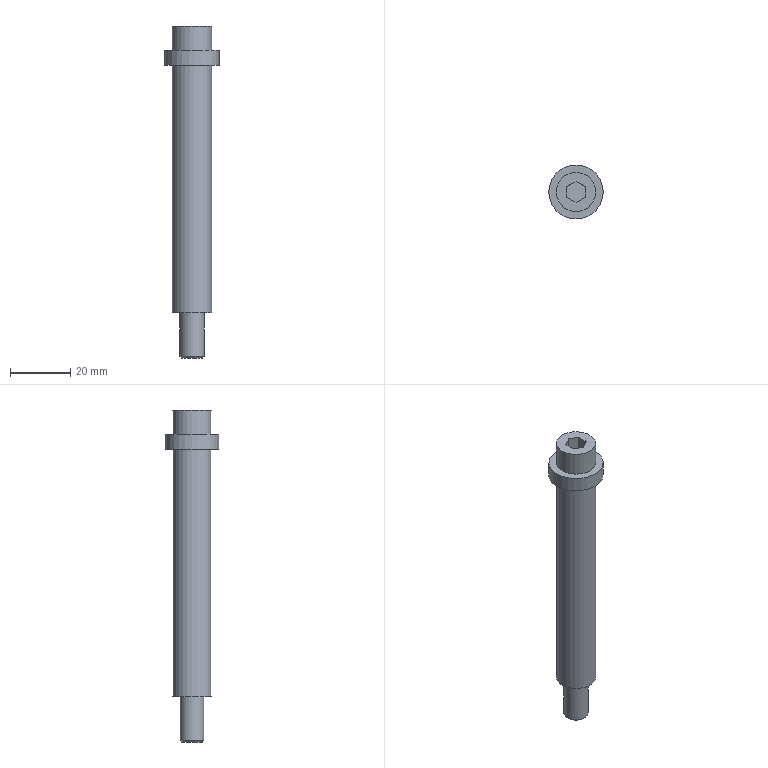Part | STEP file | gslz 2016.10.28-6_id486_x_t | 1 solid | 17 faces | box 18 x 18 x 110 mm | volume 13813 mm3 | plane 12 | cylinder 4 | cone 1 | commonest cylinder face diameters 13 x2 8 x1 18 x1
STEP:
#1=CARTESIAN_POINT('',(-78.5,245.,-15.));
#2=VERTEX_POINT('',#1);
#3=CARTESIAN_POINT('',(-75.,245.,-15.));
#4=DIRECTION('',(0.,0.,-1.));
#5=DIRECTION('',(-1.,0.,0.));
#6=AXIS2_PLACEMENT_3D('',#3,#4,#5);
#7=CIRCLE('',#6,3.5);
#8=EDGE_CURVE('',#2,#2,#7,.T.);
#9=ORIENTED_EDGE('',*,*,#8,.T.);
#10=EDGE_LOOP('',(#9));
#11=FACE_OUTER_BOUND('',#10,.T.);
#12=CARTESIAN_POINT('',(-75.,245.,-15.));
#13=DIRECTION('',(0.,0.,-1.));
#14=DIRECTION('',(1.,0.,0.));
#15=AXIS2_PLACEMENT_3D('',#12,#13,#14);
#16=PLANE('',#15);
#17=ADVANCED_FACE('',(#11),#16,.T.);
#18=CARTESIAN_POINT('',(-66.,245.,87.));
#19=VERTEX_POINT('',#18);
#20=CARTESIAN_POINT('',(-75.,245.,87.));
#21=DIRECTION('',(0.,0.,-1.));
#22=DIRECTION('',(1.,0.,0.));
#23=AXIS2_PLACEMENT_3D('',#20,#21,#22);
#24=CIRCLE('',#23,9.);
#25=EDGE_CURVE('',#19,#19,#24,.T.);
#26=ORIENTED_EDGE('',*,*,#25,.F.);
#27=EDGE_LOOP('',(#26));
#28=FACE_BOUND('',#27,.T.);
#29=CARTESIAN_POINT('',(-68.5,245.,87.));
#30=VERTEX_POINT('',#29);
#31=CARTESIAN_POINT('',(-75.,245.,87.));
#32=DIRECTION('',(0.,0.,1.));
#33=DIRECTION('',(1.,0.,0.));
#34=AXIS2_PLACEMENT_3D('',#31,#32,#33);
#35=CIRCLE('',#34,6.5);
#36=EDGE_CURVE('',#30,#30,#35,.T.);
#37=ORIENTED_EDGE('',*,*,#36,.F.);
#38=EDGE_LOOP('',(#37));
#39=FACE_BOUND('',#38,.T.);
#40=CARTESIAN_POINT('',(-75.,245.,87.));
#41=DIRECTION('',(0.,0.,1.));
#42=DIRECTION('',(-1.,0.,0.));
#43=AXIS2_PLACEMENT_3D('',#40,#41,#42);
#44=PLANE('',#43);
#45=ADVANCED_FACE('',(#28,#39),#44,.T.);
#46=ORIENTED_EDGE('',*,*,#25,.T.);
#47=EDGE_LOOP('',(#46));
#48=FACE_BOUND('',#47,.T.);
#49=CARTESIAN_POINT('',(-84.,245.,82.));
#50=VERTEX_POINT('',#49);
#51=CARTESIAN_POINT('',(-75.,245.,82.));
#52=DIRECTION('',(0.,0.,1.));
#53=DIRECTION('',(-1.,0.,0.));
#54=AXIS2_PLACEMENT_3D('',#51,#52,#53);
#55=CIRCLE('',#54,9.);
#56=EDGE_CURVE('',#50,#50,#55,.T.);
#57=ORIENTED_EDGE('',*,*,#56,.T.);
#58=EDGE_LOOP('',(#57));
#59=FACE_BOUND('',#58,.T.);
#60=CARTESIAN_POINT('',(-75.,245.,79.));
#61=DIRECTION('',(0.,0.,1.));
#62=DIRECTION('',(1.,0.,0.));
#63=AXIS2_PLACEMENT_3D('',#60,#61,#62);
#64=CYLINDRICAL_SURFACE('',#63,9.);
#65=ADVANCED_FACE('',(#48,#59),#64,.T.);
#66=CARTESIAN_POINT('',(-81.5,245.,82.));
#67=VERTEX_POINT('',#66);
#68=CARTESIAN_POINT('',(-75.,245.,82.));
#69=DIRECTION('',(0.,0.,-1.));
#70=DIRECTION('',(-1.,0.,0.));
#71=AXIS2_PLACEMENT_3D('',#68,#69,#70);
#72=CIRCLE('',#71,6.5);
#73=EDGE_CURVE('',#67,#67,#72,.T.);
#74=ORIENTED_EDGE('',*,*,#73,.F.);
#75=EDGE_LOOP('',(#74));
#76=FACE_BOUND('',#75,.T.);
#77=ORIENTED_EDGE('',*,*,#56,.F.);
#78=EDGE_LOOP('',(#77));
#79=FACE_BOUND('',#78,.T.);
#80=CARTESIAN_POINT('',(-75.,245.,82.));
#81=DIRECTION('',(0.,0.,-1.));
#82=DIRECTION('',(1.,0.,0.));
#83=AXIS2_PLACEMENT_3D('',#80,#81,#82);
#84=PLANE('',#83);
#85=ADVANCED_FACE('',(#76,#79),#84,.T.);
#86=CARTESIAN_POINT('',(-79.,245.,-14.5));
#87=VERTEX_POINT('',#86);
#88=CARTESIAN_POINT('',(-75.,245.,-14.5));
#89=DIRECTION('',(0.,0.,1.));
#90=DIRECTION('',(-1.,0.,0.));
#91=AXIS2_PLACEMENT_3D('',#88,#89,#90);
#92=CIRCLE('',#91,4.);
#93=EDGE_CURVE('',#87,#87,#92,.T.);
#94=ORIENTED_EDGE('',*,*,#93,.T.);
#95=EDGE_LOOP('',(#94));
#96=FACE_BOUND('',#95,.T.);
#97=CARTESIAN_POINT('',(-79.,245.,0.));
#98=VERTEX_POINT('',#97);
#99=CARTESIAN_POINT('',(-75.,245.,0.));
#100=DIRECTION('',(0.,0.,-1.));
#101=DIRECTION('',(-1.,0.,0.));
#102=AXIS2_PLACEMENT_3D('',#99,#100,#101);
#103=CIRCLE('',#102,4.);
#104=EDGE_CURVE('',#98,#98,#103,.T.);
#105=ORIENTED_EDGE('',*,*,#104,.T.);
#106=EDGE_LOOP('',(#105));
#107=FACE_BOUND('',#106,.T.);
#108=CARTESIAN_POINT('',(-75.,245.,0.));
#109=DIRECTION('',(0.,0.,-1.));
#110=DIRECTION('',(-1.,0.,0.));
#111=AXIS2_PLACEMENT_3D('',#108,#109,#110);
#112=CYLINDRICAL_SURFACE('',#111,4.);
#113=ADVANCED_FACE('',(#96,#107),#112,.T.);
#114=ORIENTED_EDGE('',*,*,#104,.F.);
#115=EDGE_LOOP('',(#114));
#116=FACE_BOUND('',#115,.T.);
#117=CARTESIAN_POINT('',(-81.5,245.,0.));
#118=VERTEX_POINT('',#117);
#119=CARTESIAN_POINT('',(-75.,245.,0.));
#120=DIRECTION('',(0.,0.,1.));
#121=DIRECTION('',(-1.,0.,0.));
#122=AXIS2_PLACEMENT_3D('',#119,#120,#121);
#123=CIRCLE('',#122,6.5);
#124=EDGE_CURVE('',#118,#118,#123,.T.);
#125=ORIENTED_EDGE('',*,*,#124,.F.);
#126=EDGE_LOOP('',(#125));
#127=FACE_BOUND('',#126,.T.);
#128=CARTESIAN_POINT('',(-75.,245.,0.));
#129=DIRECTION('',(0.,0.,-1.));
#130=DIRECTION('',(1.,0.,0.));
#131=AXIS2_PLACEMENT_3D('',#128,#129,#130);
#132=PLANE('',#131);
#133=ADVANCED_FACE('',(#116,#127),#132,.T.);
#134=ORIENTED_EDGE('',*,*,#73,.T.);
#135=EDGE_LOOP('',(#134));
#136=FACE_BOUND('',#135,.T.);
#137=ORIENTED_EDGE('',*,*,#124,.T.);
#138=EDGE_LOOP('',(#137));
#139=FACE_BOUND('',#138,.T.);
#140=CARTESIAN_POINT('',(-75.,245.,40.));
#141=DIRECTION('',(0.,0.,1.));
#142=DIRECTION('',(1.,0.,0.));
#143=AXIS2_PLACEMENT_3D('',#140,#141,#142);
#144=CYLINDRICAL_SURFACE('',#143,6.5);
#145=ADVANCED_FACE('',(#136,#139),#144,.T.);
#146=ORIENTED_EDGE('',*,*,#36,.T.);
#147=EDGE_LOOP('',(#146));
#148=FACE_BOUND('',#147,.T.);
#149=CARTESIAN_POINT('',(-68.5,245.,95.));
#150=VERTEX_POINT('',#149);
#151=CARTESIAN_POINT('',(-75.,245.,95.));
#152=DIRECTION('',(0.,0.,-1.));
#153=DIRECTION('',(1.,0.,0.));
#154=AXIS2_PLACEMENT_3D('',#151,#152,#153);
#155=CIRCLE('',#154,6.5);
#156=EDGE_CURVE('',#150,#150,#155,.T.);
#157=ORIENTED_EDGE('',*,*,#156,.T.);
#158=EDGE_LOOP('',(#157));
#159=FACE_BOUND('',#158,.T.);
#160=CARTESIAN_POINT('',(-75.,245.,59.));
#161=DIRECTION('',(0.,0.,1.));
#162=DIRECTION('',(1.,0.,0.));
#163=AXIS2_PLACEMENT_3D('',#160,#161,#162);
#164=CYLINDRICAL_SURFACE('',#163,6.5);
#165=ADVANCED_FACE('',(#148,#159),#164,.T.);
#166=CARTESIAN_POINT('',(-78.,246.732,90.));
#167=VERTEX_POINT('',#166);
#168=CARTESIAN_POINT('',(-78.,243.268,90.));
#169=VERTEX_POINT('',#168);
#170=CARTESIAN_POINT('',(-78.,242.691,90.));
#171=DIRECTION('',(0.,-1.,0.));
#172=VECTOR('',#171,1.);
#173=LINE('',#170,#172);
#174=EDGE_CURVE('',#167,#169,#173,.T.);
#175=ORIENTED_EDGE('',*,*,#174,.T.);
#176=CARTESIAN_POINT('',(-75.,241.536,90.));
#177=VERTEX_POINT('',#176);
#178=CARTESIAN_POINT('',(-78.5,243.557,90.));
#179=DIRECTION('',(0.866,-0.5,0.));
#180=VECTOR('',#179,1.);
#181=LINE('',#178,#180);
#182=EDGE_CURVE('',#169,#177,#181,.T.);
#183=ORIENTED_EDGE('',*,*,#182,.T.);
#184=CARTESIAN_POINT('',(-72.,243.268,90.));
#185=VERTEX_POINT('',#184);
#186=CARTESIAN_POINT('',(-77.5,240.093,90.));
#187=DIRECTION('',(0.866,0.5,0.));
#188=VECTOR('',#187,1.);
#189=LINE('',#186,#188);
#190=EDGE_CURVE('',#177,#185,#189,.T.);
#191=ORIENTED_EDGE('',*,*,#190,.T.);
#192=CARTESIAN_POINT('',(-72.,246.732,90.));
#193=VERTEX_POINT('',#192);
#194=CARTESIAN_POINT('',(-72.,242.691,90.));
#195=DIRECTION('',(0.,1.,0.));
#196=VECTOR('',#195,1.);
#197=LINE('',#194,#196);
#198=EDGE_CURVE('',#185,#193,#197,.T.);
#199=ORIENTED_EDGE('',*,*,#198,.T.);
#200=CARTESIAN_POINT('',(-75.,248.464,90.));
#201=VERTEX_POINT('',#200);
#202=CARTESIAN_POINT('',(-75.5,248.753,90.));
#203=DIRECTION('',(-0.866,0.5,0.));
#204=VECTOR('',#203,1.);
#205=LINE('',#202,#204);
#206=EDGE_CURVE('',#193,#201,#205,.T.);
#207=ORIENTED_EDGE('',*,*,#206,.T.);
#208=CARTESIAN_POINT('',(-80.5,245.289,90.));
#209=DIRECTION('',(-0.866,-0.5,0.));
#210=VECTOR('',#209,1.);
#211=LINE('',#208,#210);
#212=EDGE_CURVE('',#201,#167,#211,.T.);
#213=ORIENTED_EDGE('',*,*,#212,.T.);
#214=EDGE_LOOP('',(#175,#183,#191,#199,#207,#213));
#215=FACE_OUTER_BOUND('',#214,.T.);
#216=CARTESIAN_POINT('',(-79.,242.691,90.));
#217=DIRECTION('',(0.,0.,1.));
#218=DIRECTION('',(-1.,0.,0.));
#219=AXIS2_PLACEMENT_3D('',#216,#217,#218);
#220=PLANE('',#219);
#221=ADVANCED_FACE('',(#215),#220,.T.);
#222=CARTESIAN_POINT('',(-78.,243.268,95.));
#223=VERTEX_POINT('',#222);
#224=CARTESIAN_POINT('',(-75.,241.536,95.));
#225=VERTEX_POINT('',#224);
#226=CARTESIAN_POINT('',(-76.5,242.402,95.));
#227=DIRECTION('',(0.866,-0.5,0.));
#228=VECTOR('',#227,1.);
#229=LINE('',#226,#228);
#230=EDGE_CURVE('',#223,#225,#229,.T.);
#231=ORIENTED_EDGE('',*,*,#230,.T.);
#232=CARTESIAN_POINT('',(-75.,241.536,94.));
#233=DIRECTION('',(0.,0.,1.));
#234=VECTOR('',#233,1.);
#235=LINE('',#232,#234);
#236=EDGE_CURVE('',#177,#225,#235,.T.);
#237=ORIENTED_EDGE('',*,*,#236,.F.);
#238=ORIENTED_EDGE('',*,*,#182,.F.);
#239=CARTESIAN_POINT('',(-78.,243.268,94.));
#240=DIRECTION('',(0.,0.,1.));
#241=VECTOR('',#240,1.);
#242=LINE('',#239,#241);
#243=EDGE_CURVE('',#169,#223,#242,.T.);
#244=ORIENTED_EDGE('',*,*,#243,.T.);
#245=EDGE_LOOP('',(#231,#237,#238,#244));
#246=FACE_OUTER_BOUND('',#245,.T.);
#247=CARTESIAN_POINT('',(-78.5,243.557,94.));
#248=DIRECTION('',(-0.5,-0.866,0.));
#249=DIRECTION('',(-0.866,0.5,0.));
#250=AXIS2_PLACEMENT_3D('',#247,#248,#249);
#251=PLANE('',#250);
#252=ADVANCED_FACE('',(#246),#251,.F.);
#253=CARTESIAN_POINT('',(-72.,243.268,95.));
#254=VERTEX_POINT('',#253);
#255=CARTESIAN_POINT('',(-73.5,242.402,95.));
#256=DIRECTION('',(0.866,0.5,0.));
#257=VECTOR('',#256,1.);
#258=LINE('',#255,#257);
#259=EDGE_CURVE('',#225,#254,#258,.T.);
#260=ORIENTED_EDGE('',*,*,#259,.T.);
#261=CARTESIAN_POINT('',(-72.,243.268,94.));
#262=DIRECTION('',(0.,0.,1.));
#263=VECTOR('',#262,1.);
#264=LINE('',#261,#263);
#265=EDGE_CURVE('',#185,#254,#264,.T.);
#266=ORIENTED_EDGE('',*,*,#265,.F.);
#267=ORIENTED_EDGE('',*,*,#190,.F.);
#268=ORIENTED_EDGE('',*,*,#236,.T.);
#269=EDGE_LOOP('',(#260,#266,#267,#268));
#270=FACE_OUTER_BOUND('',#269,.T.);
#271=CARTESIAN_POINT('',(-75.5,241.247,94.));
#272=DIRECTION('',(0.5,-0.866,0.));
#273=DIRECTION('',(-0.866,-0.5,0.));
#274=AXIS2_PLACEMENT_3D('',#271,#272,#273);
#275=PLANE('',#274);
#276=ADVANCED_FACE('',(#270),#275,.F.);
#277=CARTESIAN_POINT('',(-72.,246.732,95.));
#278=VERTEX_POINT('',#277);
#279=CARTESIAN_POINT('',(-72.,245.,95.));
#280=DIRECTION('',(0.,1.,0.));
#281=VECTOR('',#280,1.);
#282=LINE('',#279,#281);
#283=EDGE_CURVE('',#254,#278,#282,.T.);
#284=ORIENTED_EDGE('',*,*,#283,.T.);
#285=CARTESIAN_POINT('',(-72.,246.732,94.));
#286=DIRECTION('',(0.,0.,1.));
#287=VECTOR('',#286,1.);
#288=LINE('',#285,#287);
#289=EDGE_CURVE('',#193,#278,#288,.T.);
#290=ORIENTED_EDGE('',*,*,#289,.F.);
#291=ORIENTED_EDGE('',*,*,#198,.F.);
#292=ORIENTED_EDGE('',*,*,#265,.T.);
#293=EDGE_LOOP('',(#284,#290,#291,#292));
#294=FACE_OUTER_BOUND('',#293,.T.);
#295=CARTESIAN_POINT('',(-72.,242.691,94.));
#296=DIRECTION('',(1.,0.,0.));
#297=DIRECTION('',(0.,0.,1.));
#298=AXIS2_PLACEMENT_3D('',#295,#296,#297);
#299=PLANE('',#298);
#300=ADVANCED_FACE('',(#294),#299,.F.);
#301=CARTESIAN_POINT('',(-75.,248.464,95.));
#302=VERTEX_POINT('',#301);
#303=CARTESIAN_POINT('',(-73.5,247.598,95.));
#304=DIRECTION('',(-0.866,0.5,0.));
#305=VECTOR('',#304,1.);
#306=LINE('',#303,#305);
#307=EDGE_CURVE('',#278,#302,#306,.T.);
#308=ORIENTED_EDGE('',*,*,#307,.T.);
#309=CARTESIAN_POINT('',(-75.,248.464,94.));
#310=DIRECTION('',(0.,0.,1.));
#311=VECTOR('',#310,1.);
#312=LINE('',#309,#311);
#313=EDGE_CURVE('',#201,#302,#312,.T.);
#314=ORIENTED_EDGE('',*,*,#313,.F.);
#315=ORIENTED_EDGE('',*,*,#206,.F.);
#316=ORIENTED_EDGE('',*,*,#289,.T.);
#317=EDGE_LOOP('',(#308,#314,#315,#316));
#318=FACE_OUTER_BOUND('',#317,.T.);
#319=CARTESIAN_POINT('',(-71.5,246.443,94.));
#320=DIRECTION('',(0.5,0.866,0.));
#321=DIRECTION('',(0.866,-0.5,0.));
#322=AXIS2_PLACEMENT_3D('',#319,#320,#321);
#323=PLANE('',#322);
#324=ADVANCED_FACE('',(#318),#323,.F.);
#325=CARTESIAN_POINT('',(-78.,246.732,95.));
#326=VERTEX_POINT('',#325);
#327=CARTESIAN_POINT('',(-76.5,247.598,95.));
#328=DIRECTION('',(-0.866,-0.5,0.));
#329=VECTOR('',#328,1.);
#330=LINE('',#327,#329);
#331=EDGE_CURVE('',#302,#326,#330,.T.);
#332=ORIENTED_EDGE('',*,*,#331,.T.);
#333=CARTESIAN_POINT('',(-78.,246.732,94.));
#334=DIRECTION('',(0.,0.,1.));
#335=VECTOR('',#334,1.);
#336=LINE('',#333,#335);
#337=EDGE_CURVE('',#167,#326,#336,.T.);
#338=ORIENTED_EDGE('',*,*,#337,.F.);
#339=ORIENTED_EDGE('',*,*,#212,.F.);
#340=ORIENTED_EDGE('',*,*,#313,.T.);
#341=EDGE_LOOP('',(#332,#338,#339,#340));
#342=FACE_OUTER_BOUND('',#341,.T.);
#343=CARTESIAN_POINT('',(-74.5,248.753,94.));
#344=DIRECTION('',(-0.5,0.866,0.));
#345=DIRECTION('',(0.866,0.5,0.));
#346=AXIS2_PLACEMENT_3D('',#343,#344,#345);
#347=PLANE('',#346);
#348=ADVANCED_FACE('',(#342),#347,.F.);
#349=CARTESIAN_POINT('',(-78.,245.,95.));
#350=DIRECTION('',(0.,-1.,0.));
#351=VECTOR('',#350,1.);
#352=LINE('',#349,#351);
#353=EDGE_CURVE('',#326,#223,#352,.T.);
#354=ORIENTED_EDGE('',*,*,#353,.T.);
#355=ORIENTED_EDGE('',*,*,#243,.F.);
#356=ORIENTED_EDGE('',*,*,#174,.F.);
#357=ORIENTED_EDGE('',*,*,#337,.T.);
#358=EDGE_LOOP('',(#354,#355,#356,#357));
#359=FACE_OUTER_BOUND('',#358,.T.);
#360=CARTESIAN_POINT('',(-78.,247.309,94.));
#361=DIRECTION('',(-1.,0.,0.));
#362=DIRECTION('',(0.,0.,-1.));
#363=AXIS2_PLACEMENT_3D('',#360,#361,#362);
#364=PLANE('',#363);
#365=ADVANCED_FACE('',(#359),#364,.F.);
#366=ORIENTED_EDGE('',*,*,#156,.F.);
#367=EDGE_LOOP('',(#366));
#368=FACE_BOUND('',#367,.T.);
#369=ORIENTED_EDGE('',*,*,#353,.F.);
#370=ORIENTED_EDGE('',*,*,#331,.F.);
#371=ORIENTED_EDGE('',*,*,#307,.F.);
#372=ORIENTED_EDGE('',*,*,#283,.F.);
#373=ORIENTED_EDGE('',*,*,#259,.F.);
#374=ORIENTED_EDGE('',*,*,#230,.F.);
#375=EDGE_LOOP('',(#369,#370,#371,#372,#373,#374));
#376=FACE_BOUND('',#375,.T.);
#377=CARTESIAN_POINT('',(-75.,245.,95.));
#378=DIRECTION('',(0.,0.,1.));
#379=DIRECTION('',(-1.,0.,0.));
#380=AXIS2_PLACEMENT_3D('',#377,#378,#379);
#381=PLANE('',#380);
#382=ADVANCED_FACE('',(#368,#376),#381,.T.);
#383=ORIENTED_EDGE('',*,*,#93,.F.);
#384=EDGE_LOOP('',(#383));
#385=FACE_BOUND('',#384,.T.);
#386=ORIENTED_EDGE('',*,*,#8,.F.);
#387=EDGE_LOOP('',(#386));
#388=FACE_BOUND('',#387,.T.);
#389=CARTESIAN_POINT('',(-75.,245.,-15.));
#390=DIRECTION('',(0.,0.,1.));
#391=DIRECTION('',(1.,0.,0.));
#392=AXIS2_PLACEMENT_3D('',#389,#390,#391);
#393=CONICAL_SURFACE('',#392,3.5,45.);
#394=ADVANCED_FACE('',(#385,#388),#393,.T.);
#395=CLOSED_SHELL('',(#17,#45,#65,#85,#113,#133,#145,#165,#221,#252,#276,#300,#324,#348,#365,#382,#394));
#396=MANIFOLD_SOLID_BREP('',#395);
#397=(LENGTH_UNIT()NAMED_UNIT(*)SI_UNIT(.MILLI.,.METRE.));
#398=UNCERTAINTY_MEASURE_WITH_UNIT(LENGTH_MEASURE(0.00002),#397,'','');
#399=(NAMED_UNIT(*)PLANE_ANGLE_UNIT()SI_UNIT($,.RADIAN.));
#400=PLANE_ANGLE_MEASURE_WITH_UNIT(PLANE_ANGLE_MEASURE(0.01745),#399);
#401=DIMENSIONAL_EXPONENTS(0.,0.,0.,0.,0.,0.,0.);
#402=(CONVERSION_BASED_UNIT('DEGREE',#400)NAMED_UNIT(#401)PLANE_ANGLE_UNIT());
#403=(NAMED_UNIT(*)SI_UNIT($,.STERADIAN.)SOLID_ANGLE_UNIT());
#404=(GEOMETRIC_REPRESENTATION_CONTEXT(3)GLOBAL_UNCERTAINTY_ASSIGNED_CONTEXT((#398))GLOBAL_UNIT_ASSIGNED_CONTEXT((#397,#402,#403))REPRESENTATION_CONTEXT('',''));
#405=ADVANCED_BREP_SHAPE_REPRESENTATION('',(#396),#404);